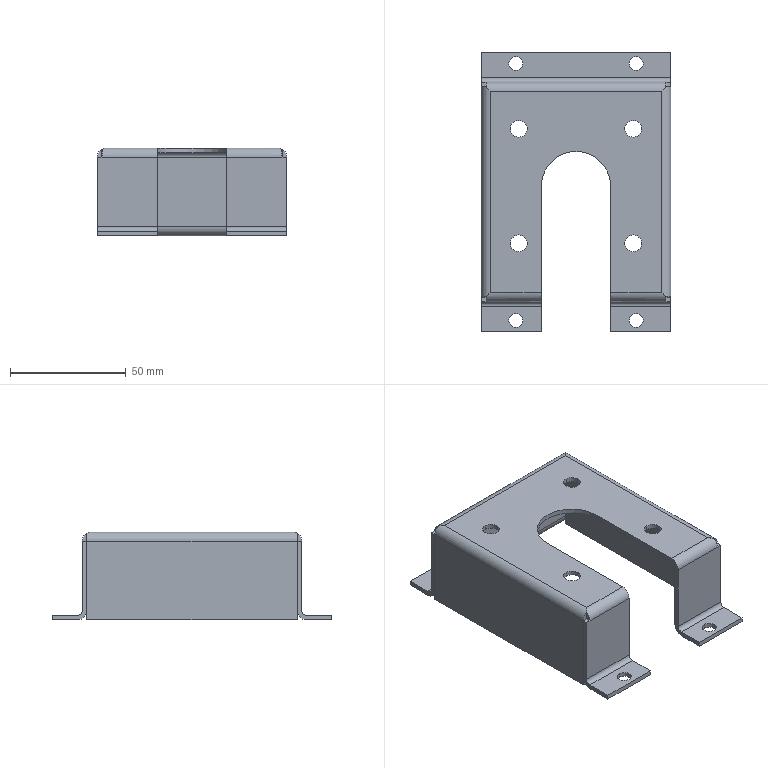Part | NX | features solid 2 | 1 solid | 82 faces | box 82 x 121 x 38 mm | volume 36320 mm3 | plane 49 | cylinder 33 | commonest cylinder face diameters 4 x8 6 x8 7.2 x8 8 x8 30 x1